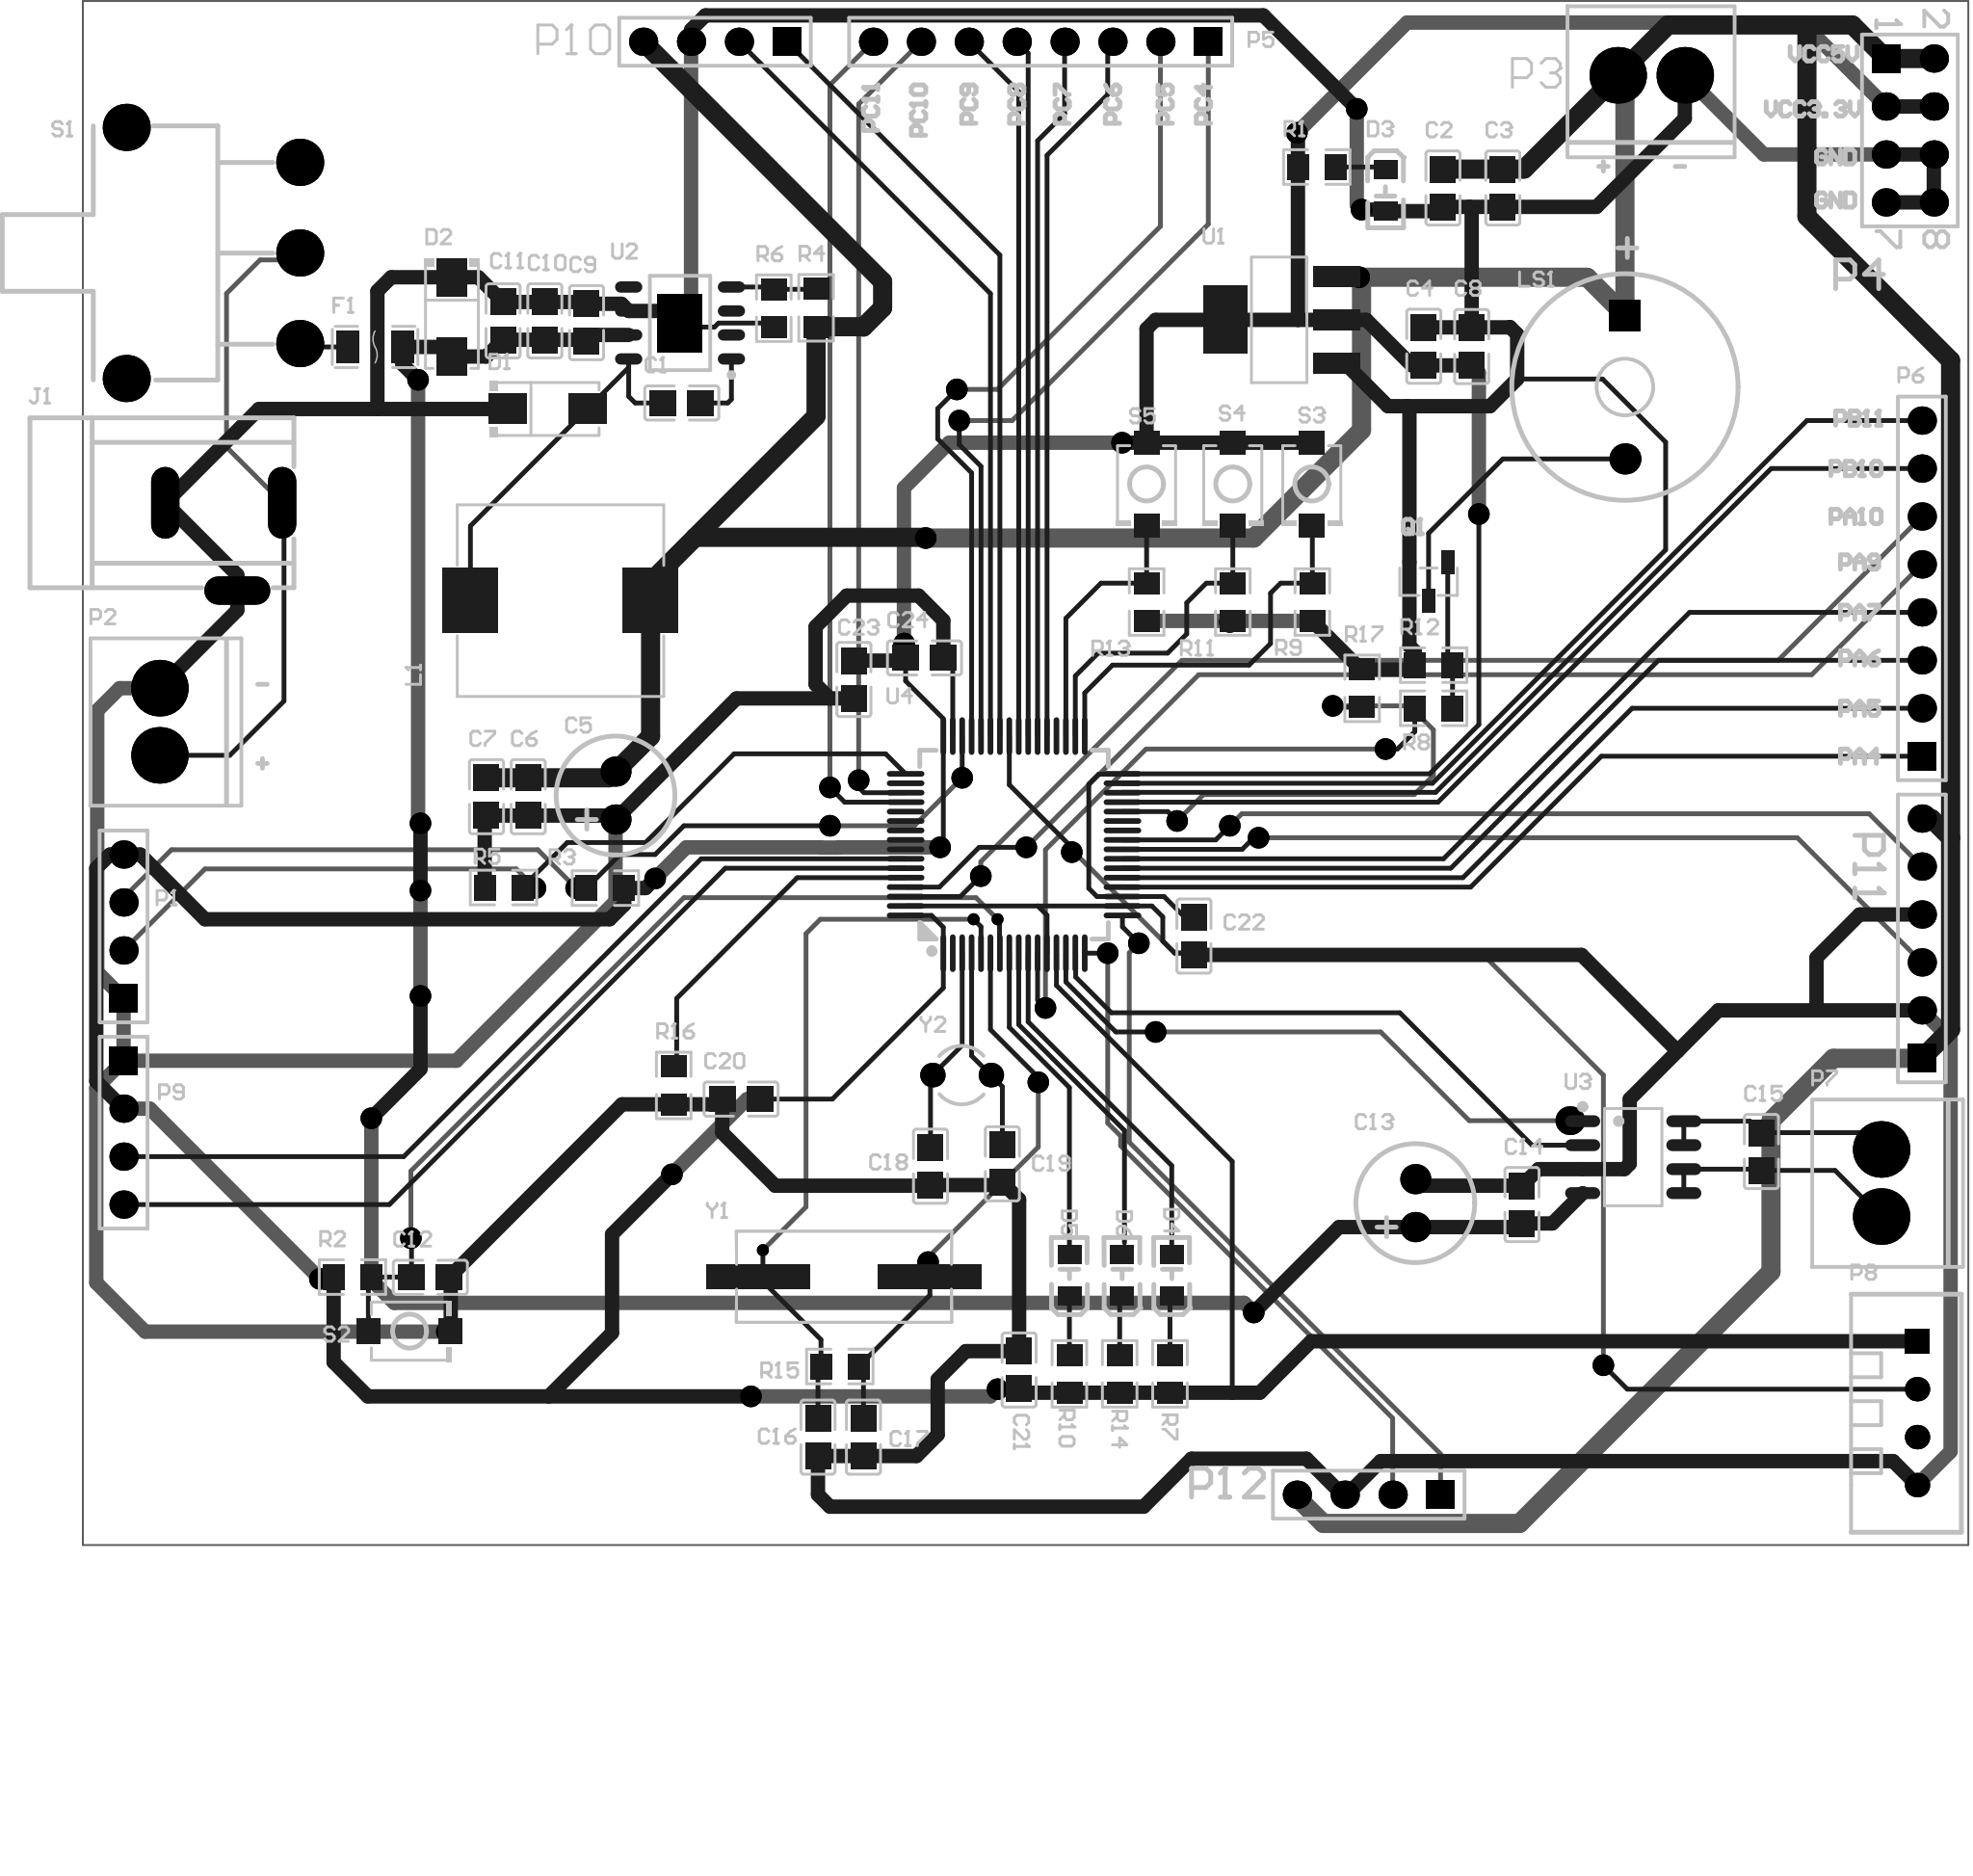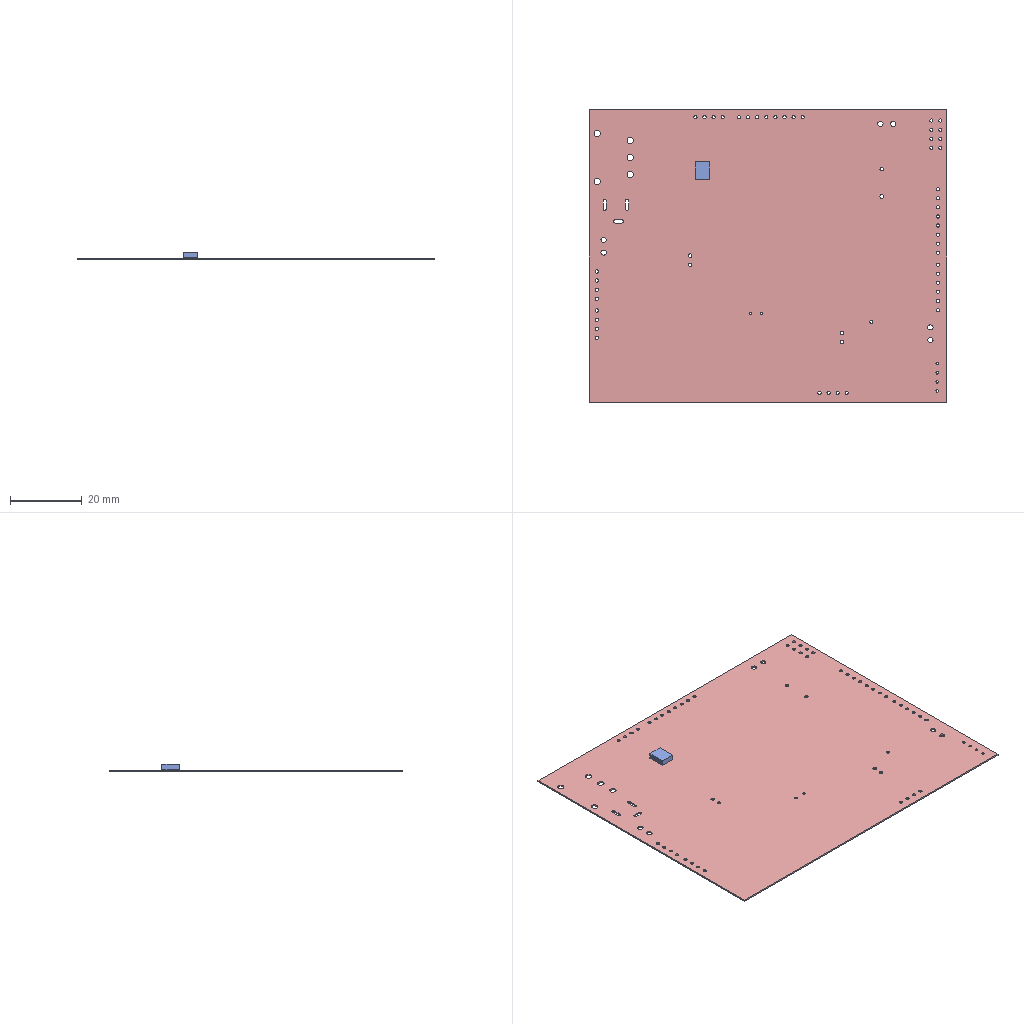Circuit board layout | Altium Designer | box 100 x 81.8 x 2.1 mm
Layer stack:
# Altium Designer layer stack of  (unit mm; dielectric type: 0 none, 1 core, 2 prepreg, 3 surface material)
index,name,kind,layer,copper_thickness_mm,dielectric_type,dielectric_thickness_mm,dielectric_material,dielectric_constant
0,Top Paste,other,,,,,,
1,Top Overlay,other,,,,,,
2,Top Solder,dielectric,,,3,0.0102,Solder Resist,3.5
3,Top Layer,copper,Top Layer,0.0356,,,,
4,Dielectric 1,dielectric,,,0,0.32,FR-4,4.8
5,Bottom Layer,copper,Bottom Layer,0.0356,,,,
6,Bottom Solder,dielectric,,,3,0.0102,Solder Resist,3.5
7,Bottom Overlay,other,,,,,,
8,Bottom Paste,other,,,,,,
# drill layer pairs: low layer,high layer
drill_pair,Top Layer,Bottom Layer
Part placement:
Designator,Comment,Layer,Footprint,Center-X(mm),Center-Y(mm),Rotation
C2,10uF,TopLayer,C0805,97.663,116.967,90
C3,0.1uF,TopLayer,C0805,100.838,116.967,90
C4,10uF,TopLayer,C0805,96.647,108.585,270
C5,330uF/16V,TopLayer,220uF,53.779,84.786,90
C6,0.1uF,TopLayer,C0805,49.149,84.725,90
C7,0.01uF,TopLayer,C0805,46.935,84.725,90
C8,0.1uF,TopLayer,C0805,99.187,108.569,270
C9,10uF/25V,TopLayer,C0805,52.242,109.834,270
C10,10uF/25V,TopLayer,C0805,50.028,109.929,270
C11,0.01uF,TopLayer,C0805,47.814,109.929,270
C1,0.01uF,TopLayer,C0805,57.293,105.579,180
C12,0.1uF,TopLayer,C0805,43.958,59.267,360
C16,22pF,TopLayer,C0805,64.516,50.8,270
C17,22pF,TopLayer,C0805,66.929,50.8,270
C13,220uF/16V,TopLayer,220uF,96.197,63.196,90
C14,0.01uF,TopLayer,C0805,101.854,63.119,90
C15,0.01uF,TopLayer,C0805,114.554,65.929,90
C18,15pF,TopLayer,C0805,70.485,65.151,90
C19,15pF,TopLayer,C0805,74.295,65.278,270
C20,0.1uF,TopLayer,C0805,60.436,68.707,180
C21,0.1uF,TopLayer,C0805,75.184,54.356,90
C22,0.1uF,TopLayer,C0805,84.455,77.343,270
C23,0.1uF,TopLayer,C0805,66.421,90.932,270
C24,0.1uF,TopLayer,C0805,70.164,92.075,360
D1,SS54,TopLayer,SMA,50.178,105.26,360
D2,SMBJ12A,TopLayer,SMA,45.103,110.14,270
D3,LED0,TopLayer,LED0805-RD_RED,94.615,116.84,270
D4,LED0,TopLayer,LED0805-RD_RED,83.279,59.393,90
D5,LED0,TopLayer,LED0805-RD_RED,77.851,59.393,90
D6,LED0,TopLayer,LED0805-RD_RED,80.645,59.393,90
F1,3A/16V,TopLayer,C70065,41.026,108.548,360
J1,DC-jack3,TopLayer,SANJIAO,32.998,97.968,90
L1,Inductor,TopLayer,DIANGAN,50.861,95.11,180
LS1,Speaker,TopLayer,BZ,107.315,106.426,270
P1,Header 4,TopLayer,HDR1X4,27.686,77.851,90
P7,Header 2,TopLayer,KF350,120.904,64.262,180
P8,DHT11,TopLayer,DHT11,122.809,52.07,270
P9,Header 4,TopLayer,HDR1X4,27.686,66.929,270
P10,HC-06,TopLayer,HDR1X4,59.055,124.714,180
P5,Header 8,TopLayer,HDR1X8,76.327,124.714,180
P6,Header 8,TopLayer,HDR1X8,123.063,95.758,90
R1,10K,TopLayer,R0805,90.972,118.079,180
R2,10K,TopLayer,R0805,39.827,59.28,180
R3,10K,TopLayer,R0805,53.242,79.883,180
R4,10K,TopLayer,R0805,64.415,110.62,270
R5,10K,TopLayer,R0805,47.839,79.914,360
R6,3.16K,TopLayer,R0805,62.174,110.601,90
R7,10K,TopLayer,R0805,83.185,54.154,270
R9,10K,TopLayer,R0805,90.736,95.036,270
R10,10K,TopLayer,R0805,77.851,54.154,270
R11,10K,TopLayer,R0805,86.518,95.036,270
R13,10K,TopLayer,R0805,81.946,95.036,270
R14,10K,TopLayer,R0805,80.518,54.154,270
R15,1M,TopLayer,R0805,65.675,54.543,180
R16,10K,TopLayer,R0805,56.865,69.429,90
R8,1K,TopLayer,R0805,97.171,89.408,0
R12,10K,TopLayer,R0805,97.171,91.694,0
R17,10K,TopLayer,R0805,93.376,90.464,270
S1,SW-SPDT,TopLayer,SW-TH,32.43,113.527,90
S2,SW-PB,TopLayer,KAIGUAN,42.854,56.415,360
S3,SW-PB,TopLayer,KAIGUAN,90.705,101.291,270
S4,SW-PB,TopLayer,KAIGUAN,86.514,101.291,270
S5,SW-PB,TopLayer,KAIGUAN,81.942,101.291,270
U1,AMS1117,TopLayer,SOT-89,89.076,109.982,360
U2,TPS5450,TopLayer,CYF-SOIC-H,57.201,109.818,180
U4,stm32f103r,TopLayer,LQFP-64,74.914,82.185,0
U3,RZ7889,TopLayer,SOP-8,107.755,65.631,270
Y1,8MHz,TopLayer,JINGZHEN,65.898,59.296,180
Y2,32.768KHz,TopLayer,R38,72.136,69.977,270
P2,Header 2,TopLayer,KF350,29.591,88.694,180
P3,Header 2,TopLayer,KF350,108.712,122.936,90
Q1,NPN,TopLayer,QNPN,96.901,96.139,90
P4,Header 4X2,TopLayer,HDR2X4,122.428,120.015,270
P11,GP2Y1010AU0F,TopLayer,HDR1X6,123.063,77.216,90
P12,JW01,TopLayer,HDR1X4,93.726,47.752,180
Pad and via stacks:
# Altium Designer via and pad stacks of  (unit mm). Each distinct definition once, with the count of objects using it.
# via: kind,start_layer,end_layer,hole_mm,diameter_mm,mode(0 simple;1 top-mid-bottom;2 full stack),diameter_per_layer,count,example_net
# pad: kind,layer,hole_mm,hole_type(0 round;1 square;2 slot),plating,top_size,top_shape(1 round;2 rect;3 octagon;9 rounded rect),mid_size,bottom_size,mode,footprint,size_per_layer,count,example
pad,Top Layer,0,0,plated,1.41x1.35,2,1.41x1.35,1.41x1.35,0,C0805,,44,C22.1
pad,Top Layer,0,0,plated,2x1.593,2,2x1.593,2x1.593,0,SMA,,4,D1.2
pad,Top Layer,0,0,plated,1x1.25,2,1x1.25,1x1.25,0,LED0805-RD_RED,,8,D3.2
pad,Top Layer,0,0,plated,1.19x1.728,2,1.19x1.728,1.19x1.728,0,C70065,,2,F1.1
pad,Top Layer,0,0,plated,2.924x3.42,2,2.924x3.42,2.924x3.42,0,DIANGAN,,2,L1.2
pad,Top Layer,0,0,plated,1.133x1.377,2,1.133x1.377,1.133x1.377,0,R0805,,34,R1.2
pad,Top Layer,0,0,plated,1.23x1.36,2,1.23x1.36,1.23x1.36,0,KAIGUAN,,8,S2.1
pad,Top Layer,0,0,plated,2.5x1.1,2,2.5x1.1,2.5x1.1,0,SOT-89,,3,U1.1
pad,Top Layer,0,0,plated,2.34x3.6,2,2.34x3.6,2.34x3.6,0,SOT-89,,1,U1.2
pad,Top Layer,0,0,plated,0.6x1.45,1,0.6x1.45,0.6x1.45,0,CYF-SOIC-H,,8,U2.1
pad,Top Layer,0,0,plated,5.5x1.3,2,5.5x1.3,5.5x1.3,0,JINGZHEN,,2,Y1.2
pad,Top Layer,0,0,plated,1.25x0.7,2,1.25x0.7,1.25x0.7,0,QNPN,,3,Q1.2
pad,Top Layer,0,0,plated,0.63x1.865,1,0.63x1.865,0.63x1.865,0,SOP-8,,8,U3.5
pad,Top Layer,0,0,plated,0.3x2,1,0.3x2,0.3x2,0,LQFP-64,,32,U4.1
pad,Top Layer,0,0,plated,2x0.3,1,2x0.3,2x0.3,0,LQFP-64,,32,U4.17
pad,Multi-Layer,0.889,0,plated,1.524x1.524,1,1.524x1.524,1.524x1.524,0,,,1,3
pad,Multi-Layer,0.9,0,plated,1.5x1.5,2,1.5x1.5,1.5x1.5,0,HDR1X8,,2,P5.1
pad,Multi-Layer,0.9,0,plated,1.5x1.5,1,1.5x1.5,1.5x1.5,0,HDR1X8,,14,P5.2
pad,Multi-Layer,0.9,0,plated,1.5x1.5,1,1.5x1.5,1.5x1.5,0,HDR1X4,,12,P9.4
pad,Multi-Layer,0.9,0,plated,1.5x1.5,2,1.5x1.5,1.5x1.5,0,HDR1X4,,4,P9.1
pad,Multi-Layer,1,0,plated,1.65x1.65,1,1.65x1.65,1.65x1.65,0,BZ,,1,LS1.2
pad,Multi-Layer,1,0,plated,1.65x1.65,2,1.65x1.65,1.65x1.65,0,BZ,,1,LS1.1
pad,Multi-Layer,1,0,plated,1.6x1.6,1,1.6x1.6,1.6x1.6,0,220uF,,4,C5.1
pad,Multi-Layer,0.9,2,plated,1.5x3.8,1,1.5x3.8,1.5x3.8,0,SANJIAO,,2,J1.1
pad,Multi-Layer,0.9,2,plated,1.5x3.5,1,1.5x3.5,1.5x3.5,0,SANJIAO,,1,J1.3
pad,Multi-Layer,1.8,0,plated,2.5x2.5,1,2.5x2.5,2.5x2.5,0,SW-TH,,5,S1.1
pad,Multi-Layer,2.2,0,plated,2.4x3.1,2,2.4x3.1,2.4x3.1,0,CYF-SOIC-H,,1,U2.9
pad,Multi-Layer,0.7,0,plated,1.3x1.3,1,1.3x1.3,1.3x1.3,0,R38,,2,Y2.2
pad,Multi-Layer,1.5,0,plated,3x3,1,3x3,3x3,0,KF350,,6,P2.1
pad,Multi-Layer,0.7112,0,plated,1.295x1.295,1,1.295x1.295,1.295x1.295,0,DHT11,,3,P8.4
pad,Multi-Layer,0.7112,0,plated,1.295x1.295,2,1.295x1.295,1.295x1.295,0,DHT11,,1,P8.1
pad,Multi-Layer,0.9,0,plated,1.5x1.5,1,1.5x1.5,1.5x1.5,0,HDR2X4,,7,P4.8
pad,Multi-Layer,0.9,0,plated,1.5x1.5,2,1.5x1.5,1.5x1.5,0,HDR2X4,,1,P4.1
pad,Multi-Layer,0.9,0,plated,1.5x1.5,1,1.5x1.5,1.5x1.5,0,HDR1X6,,5,P11.6
pad,Multi-Layer,0.9,0,plated,1.5x1.5,2,1.5x1.5,1.5x1.5,0,HDR1X6,,1,P11.1
via,Top Layer,Bottom Layer,0.635,1.143,0,,50,DC IN
via,Top Layer,Bottom Layer,0.381,0.635,0,,3,NetC16_1
Design rules, without the lines most boards share:
# Altium Designer design rules of  (exported by Altium Designer, unit mm)
# columns: name | kind | enabled | priority | scope1 | scope2 | descriptor | typed fields (field=value)
Clearance | 0 | enabled | 1 | All | All | Clearance Constraint (Gap=8mil) (All),(All) | gap=0.2032
PlaneConnect | 6 | enabled | 1 | All | All | Power Plane Connect Rule(Relief Connect )(Expansion=20mil) (Conductor Width=10mil) (Air Gap=10mil) (Entries=4) (All) | relief_conductor_width=0.254 relief_entries=4 relief_expansion=0.508
PolygonConnect | 20 | enabled | 1 | All | All | Polygon Connect Rule(Relief Connect )(Conductor Width=10mil) (Relief Angle=90 Angle) (Entries=4) (Air Gap Width=10mil) (All),(All) | connect_style(0=relief,1=direct,2=none)=0 relief_conductor_width=0.254 relief_entries=4
Width | 2 | enabled | 1 | All | All | Width Constraint (Min=8mil) (Max=120mil) (Preferred=10mil) (All) |
RoutingVias | 11 | enabled | 1 | All | All | Routing Via (MinHoleWidth=12mil) (MaxHoleWidth=28mil) (PreferredHoleWidth=20mil) (MinWidth=24mil) (MaxWidth=50mil) (PreferedWidth=30mil) (All) | via_min_hole=0.3048 via_max_hole=0.7112 via_preferred_diameter=0.762 via_preferred_hole=0.508
PasteMaskExpansion | 14 | enabled | 1 | All | All | Paste Mask Expansion (Expansion =0mil) (All) | expansion=0
SolderMaskExpansion | 13 | enabled | 1 | All | All | Solder Mask Expansion (Expansion =4mil) (All) | expansion=0.1016
HoleSize | 42 | enabled | 1 | All | All | Hole Size Constraint (Min=1mil) (Max=200mil) (All) |
DiffPairsRouting | 51 | enabled | 1 | All | All | Differential Pairs Uncoupled Length using the Gap Constraints (Min=10mil) (Max=10mil) (Prefered=10mil)  and Width Constraints (Min=15mil) (Max=15mil) (Prefered=15mil) (All) |
HoleToHoleClearance | 52 | enabled | 1 | All | All | Hole To Hole Clearance (Gap=10mil) (All),(All) | gap=0.254
Classes set for this board:
# Altium Designer classes of  (member kind: 0 net, 1 component, 2 from-to, 3 pad, 4 layer, 5 differential pair, 6 design channel, 7 polygon, 8 structure, 9 xSignal)
# columns: class name | member kind | superclass | members
Sheet1 | 1 | no | C1; C2; C3; C4; C5; C6; C7; C8; C9; C10; C11; C12; C18; D1; D2; D3; D4; F1; J1; L1; LS1; P1; P2; P3; P7; P8; P9; P10; P12; Q1; R1; R2; R3; R4; R5; R6; S1; S2; S3; S4; S5; U1; U2; U4; Y1; Y2; C13; C15; C17; C14; P4; R8; R9; R11; R12; R14; R15; C16; C19; C20; C21; C22; C23; C24; D5; D6; P5; P6; P11; R7; R10; R13; R16; R17; U3;